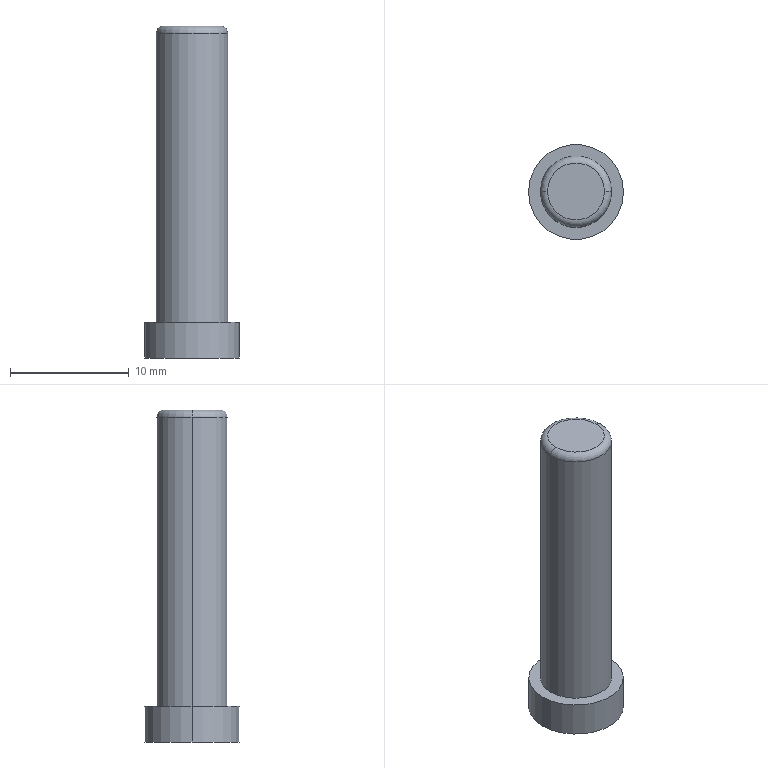Part | SolidWorks | features BaseBody 1 | 1 solid | 9 faces | box 8 x 8 x 28 mm | volume 856.499 mm3 | cylinder 4 | plane 3 | torus 2 | commonest cylinder face diameters 6.001 x2 8 x2
STEP:
#1=CARTESIAN_POINT('',(-82.,-25.,-3.829));
#2=VERTEX_POINT('',#1);
#3=CARTESIAN_POINT('',(-90.,-25.,-3.829));
#4=VERTEX_POINT('',#3);
#5=CARTESIAN_POINT('',(-86.,-25.,-3.829));
#6=DIRECTION('',(0.,0.,-1.));
#7=DIRECTION('',(1.,0.,0.));
#8=AXIS2_PLACEMENT_3D('',#5,#6,#7);
#9=CIRCLE('',#8,4.);
#10=EDGE_CURVE('',#2,#4,#9,.T.);
#11=ORIENTED_EDGE('',*,*,#10,.T.);
#12=CARTESIAN_POINT('',(-90.,-25.,-6.829));
#13=VERTEX_POINT('',#12);
#14=CARTESIAN_POINT('',(-90.,-25.,-3.829));
#15=DIRECTION('',(0.,0.,-1.));
#16=VECTOR('',#15,1000.);
#17=LINE('',#14,#16);
#18=EDGE_CURVE('',#4,#13,#17,.T.);
#19=ORIENTED_EDGE('',*,*,#18,.T.);
#20=CARTESIAN_POINT('',(-82.,-25.,-6.829));
#21=VERTEX_POINT('',#20);
#22=CARTESIAN_POINT('',(-86.,-25.,-6.829));
#23=DIRECTION('',(0.,0.,1.));
#24=DIRECTION('',(1.,0.,0.));
#25=AXIS2_PLACEMENT_3D('',#22,#23,#24);
#26=CIRCLE('',#25,4.);
#27=EDGE_CURVE('',#13,#21,#26,.T.);
#28=ORIENTED_EDGE('',*,*,#27,.T.);
#29=CARTESIAN_POINT('',(-82.,-25.,-3.829));
#30=DIRECTION('',(0.,0.,-1.));
#31=VECTOR('',#30,1000.);
#32=LINE('',#29,#31);
#33=EDGE_CURVE('',#2,#21,#32,.T.);
#34=ORIENTED_EDGE('',*,*,#33,.F.);
#35=EDGE_LOOP('',(#11,#19,#28,#34));
#36=FACE_OUTER_BOUND('',#35,.T.);
#37=CARTESIAN_POINT('',(-86.,-25.,-3.829));
#38=DIRECTION('',(0.,0.,-1.));
#39=DIRECTION('',(1.,0.,0.));
#40=AXIS2_PLACEMENT_3D('',#37,#38,#39);
#41=CYLINDRICAL_SURFACE('',#40,4.);
#42=ADVANCED_FACE('',(#36),#41,.T.);
#43=CARTESIAN_POINT('',(-89.001,-25.,20.571));
#44=VERTEX_POINT('',#43);
#45=CARTESIAN_POINT('',(-82.999,-25.,20.571));
#46=VERTEX_POINT('',#45);
#47=CARTESIAN_POINT('',(-86.,-25.,20.571));
#48=DIRECTION('',(0.,0.,-1.));
#49=DIRECTION('',(1.,0.,0.));
#50=AXIS2_PLACEMENT_3D('',#47,#48,#49);
#51=CIRCLE('',#50,3.001);
#52=EDGE_CURVE('',#44,#46,#51,.T.);
#53=ORIENTED_EDGE('',*,*,#52,.F.);
#54=CARTESIAN_POINT('',(-88.4,-25.,21.171));
#55=VERTEX_POINT('',#54);
#56=CARTESIAN_POINT('',(-88.4,-25.,20.571));
#57=DIRECTION('',(0.,1.,0.));
#58=DIRECTION('',(-1.,0.,0.));
#59=AXIS2_PLACEMENT_3D('',#56,#57,#58);
#60=CIRCLE('',#59,0.6001);
#61=EDGE_CURVE('',#44,#55,#60,.T.);
#62=ORIENTED_EDGE('',*,*,#61,.T.);
#63=CARTESIAN_POINT('',(-83.6,-25.,21.171));
#64=VERTEX_POINT('',#63);
#65=CARTESIAN_POINT('',(-86.,-25.,21.171));
#66=DIRECTION('',(0.,0.,1.));
#67=DIRECTION('',(1.,0.,0.));
#68=AXIS2_PLACEMENT_3D('',#65,#66,#67);
#69=CIRCLE('',#68,2.4);
#70=EDGE_CURVE('',#64,#55,#69,.T.);
#71=ORIENTED_EDGE('',*,*,#70,.F.);
#72=CARTESIAN_POINT('',(-83.6,-25.,20.571));
#73=DIRECTION('',(0.,-1.,0.));
#74=DIRECTION('',(0.,0.,-1.));
#75=AXIS2_PLACEMENT_3D('',#72,#73,#74);
#76=CIRCLE('',#75,0.6001);
#77=EDGE_CURVE('',#46,#64,#76,.T.);
#78=ORIENTED_EDGE('',*,*,#77,.F.);
#79=EDGE_LOOP('',(#53,#62,#71,#78));
#80=FACE_OUTER_BOUND('',#79,.T.);
#81=CARTESIAN_POINT('',(-86.,-25.,20.571));
#82=DIRECTION('',(0.,0.,1.));
#83=DIRECTION('',(1.,0.,0.));
#84=AXIS2_PLACEMENT_3D('',#81,#82,#83);
#85=TOROIDAL_SURFACE('',#84,2.4,0.6001);
#86=ADVANCED_FACE('',(#80),#85,.T.);
#87=CARTESIAN_POINT('',(-86.,-25.,20.571));
#88=DIRECTION('',(0.,0.,-1.));
#89=DIRECTION('',(1.,0.,0.));
#90=AXIS2_PLACEMENT_3D('',#87,#88,#89);
#91=CIRCLE('',#90,3.001);
#92=EDGE_CURVE('',#46,#44,#91,.T.);
#93=ORIENTED_EDGE('',*,*,#92,.T.);
#94=CARTESIAN_POINT('',(-89.001,-25.,-3.829));
#95=VERTEX_POINT('',#94);
#96=CARTESIAN_POINT('',(-89.001,-25.,21.171));
#97=DIRECTION('',(0.,0.,-1.));
#98=VECTOR('',#97,1000.);
#99=LINE('',#96,#98);
#100=EDGE_CURVE('',#44,#95,#99,.T.);
#101=ORIENTED_EDGE('',*,*,#100,.T.);
#102=CARTESIAN_POINT('',(-82.999,-25.,-3.829));
#103=VERTEX_POINT('',#102);
#104=CARTESIAN_POINT('',(-86.,-25.,-3.829));
#105=DIRECTION('',(0.,0.,1.));
#106=DIRECTION('',(1.,0.,0.));
#107=AXIS2_PLACEMENT_3D('',#104,#105,#106);
#108=CIRCLE('',#107,3.001);
#109=EDGE_CURVE('',#95,#103,#108,.T.);
#110=ORIENTED_EDGE('',*,*,#109,.T.);
#111=CARTESIAN_POINT('',(-82.999,-25.,21.171));
#112=DIRECTION('',(0.,0.,-1.));
#113=VECTOR('',#112,1000.);
#114=LINE('',#111,#113);
#115=EDGE_CURVE('',#46,#103,#114,.T.);
#116=ORIENTED_EDGE('',*,*,#115,.F.);
#117=EDGE_LOOP('',(#93,#101,#110,#116));
#118=FACE_OUTER_BOUND('',#117,.T.);
#119=CARTESIAN_POINT('',(-86.,-25.,21.171));
#120=DIRECTION('',(0.,0.,-1.));
#121=DIRECTION('',(1.,0.,0.));
#122=AXIS2_PLACEMENT_3D('',#119,#120,#121);
#123=CYLINDRICAL_SURFACE('',#122,3.001);
#124=ADVANCED_FACE('',(#118),#123,.T.);
#125=ORIENTED_EDGE('',*,*,#70,.T.);
#126=CARTESIAN_POINT('',(-86.,-25.,21.171));
#127=DIRECTION('',(0.,0.,1.));
#128=DIRECTION('',(1.,0.,0.));
#129=AXIS2_PLACEMENT_3D('',#126,#127,#128);
#130=CIRCLE('',#129,2.4);
#131=EDGE_CURVE('',#55,#64,#130,.T.);
#132=ORIENTED_EDGE('',*,*,#131,.T.);
#133=EDGE_LOOP('',(#125,#132));
#134=FACE_OUTER_BOUND('',#133,.T.);
#135=CARTESIAN_POINT('',(-86.,-25.,21.171));
#136=DIRECTION('',(0.,0.,1.));
#137=DIRECTION('',(1.,0.,0.));
#138=AXIS2_PLACEMENT_3D('',#135,#136,#137);
#139=PLANE('',#138);
#140=ADVANCED_FACE('',(#134),#139,.T.);
#141=ORIENTED_EDGE('',*,*,#100,.F.);
#142=ORIENTED_EDGE('',*,*,#52,.T.);
#143=ORIENTED_EDGE('',*,*,#115,.T.);
#144=CARTESIAN_POINT('',(-86.,-25.,-3.829));
#145=DIRECTION('',(0.,0.,1.));
#146=DIRECTION('',(1.,0.,0.));
#147=AXIS2_PLACEMENT_3D('',#144,#145,#146);
#148=CIRCLE('',#147,3.001);
#149=EDGE_CURVE('',#103,#95,#148,.T.);
#150=ORIENTED_EDGE('',*,*,#149,.T.);
#151=EDGE_LOOP('',(#141,#142,#143,#150));
#152=FACE_OUTER_BOUND('',#151,.T.);
#153=CARTESIAN_POINT('',(-86.,-25.,21.171));
#154=DIRECTION('',(0.,0.,-1.));
#155=DIRECTION('',(1.,0.,0.));
#156=AXIS2_PLACEMENT_3D('',#153,#154,#155);
#157=CYLINDRICAL_SURFACE('',#156,3.001);
#158=ADVANCED_FACE('',(#152),#157,.T.);
#159=ORIENTED_EDGE('',*,*,#61,.F.);
#160=ORIENTED_EDGE('',*,*,#92,.F.);
#161=ORIENTED_EDGE('',*,*,#77,.T.);
#162=ORIENTED_EDGE('',*,*,#131,.F.);
#163=EDGE_LOOP('',(#159,#160,#161,#162));
#164=FACE_OUTER_BOUND('',#163,.T.);
#165=CARTESIAN_POINT('',(-86.,-25.,20.571));
#166=DIRECTION('',(0.,0.,1.));
#167=DIRECTION('',(1.,0.,0.));
#168=AXIS2_PLACEMENT_3D('',#165,#166,#167);
#169=TOROIDAL_SURFACE('',#168,2.4,0.6001);
#170=ADVANCED_FACE('',(#164),#169,.T.);
#171=CARTESIAN_POINT('',(-86.,-25.,-6.829));
#172=DIRECTION('',(0.,0.,1.));
#173=DIRECTION('',(1.,0.,0.));
#174=AXIS2_PLACEMENT_3D('',#171,#172,#173);
#175=CIRCLE('',#174,4.);
#176=EDGE_CURVE('',#21,#13,#175,.T.);
#177=ORIENTED_EDGE('',*,*,#176,.F.);
#178=ORIENTED_EDGE('',*,*,#27,.F.);
#179=EDGE_LOOP('',(#177,#178));
#180=FACE_OUTER_BOUND('',#179,.T.);
#181=CARTESIAN_POINT('',(-86.,-25.,-6.829));
#182=DIRECTION('',(0.,0.,-1.));
#183=DIRECTION('',(-1.,0.,0.));
#184=AXIS2_PLACEMENT_3D('',#181,#182,#183);
#185=PLANE('',#184);
#186=ADVANCED_FACE('',(#180),#185,.T.);
#187=ORIENTED_EDGE('',*,*,#149,.F.);
#188=ORIENTED_EDGE('',*,*,#109,.F.);
#189=EDGE_LOOP('',(#187,#188));
#190=FACE_BOUND('',#189,.T.);
#191=ORIENTED_EDGE('',*,*,#10,.F.);
#192=CARTESIAN_POINT('',(-86.,-25.,-3.829));
#193=DIRECTION('',(0.,0.,-1.));
#194=DIRECTION('',(1.,0.,0.));
#195=AXIS2_PLACEMENT_3D('',#192,#193,#194);
#196=CIRCLE('',#195,4.);
#197=EDGE_CURVE('',#4,#2,#196,.T.);
#198=ORIENTED_EDGE('',*,*,#197,.F.);
#199=EDGE_LOOP('',(#191,#198));
#200=FACE_OUTER_BOUND('',#199,.T.);
#201=CARTESIAN_POINT('',(-86.,-25.,-3.829));
#202=DIRECTION('',(0.,0.,1.));
#203=DIRECTION('',(1.,0.,0.));
#204=AXIS2_PLACEMENT_3D('',#201,#202,#203);
#205=PLANE('',#204);
#206=ADVANCED_FACE('',(#190,#200),#205,.T.);
#207=ORIENTED_EDGE('',*,*,#18,.F.);
#208=ORIENTED_EDGE('',*,*,#197,.T.);
#209=ORIENTED_EDGE('',*,*,#33,.T.);
#210=ORIENTED_EDGE('',*,*,#176,.T.);
#211=EDGE_LOOP('',(#207,#208,#209,#210));
#212=FACE_OUTER_BOUND('',#211,.T.);
#213=CARTESIAN_POINT('',(-86.,-25.,-3.829));
#214=DIRECTION('',(0.,0.,-1.));
#215=DIRECTION('',(1.,0.,0.));
#216=AXIS2_PLACEMENT_3D('',#213,#214,#215);
#217=CYLINDRICAL_SURFACE('',#216,4.);
#218=ADVANCED_FACE('',(#212),#217,.T.);
#219=CLOSED_SHELL('',(#42,#86,#124,#140,#158,#170,#186,#206,#218));
#220=MANIFOLD_SOLID_BREP('',#219);
#221=CARTESIAN_POINT('',(0.,0.,0.));
#222=DIRECTION('',(0.,0.,1.));
#223=DIRECTION('',(1.,0.,0.));
#224=AXIS2_PLACEMENT_3D('',#221,#222,#223);
#225=(LENGTH_UNIT()NAMED_UNIT(*)SI_UNIT(.MILLI.,.METRE.));
#226=UNCERTAINTY_MEASURE_WITH_UNIT(LENGTH_MEASURE(0.00001),#225,'','');
#227=(NAMED_UNIT(*)PLANE_ANGLE_UNIT()SI_UNIT($,.RADIAN.));
#228=(NAMED_UNIT(*)SI_UNIT($,.STERADIAN.)SOLID_ANGLE_UNIT());
#229=(GEOMETRIC_REPRESENTATION_CONTEXT(3)GLOBAL_UNCERTAINTY_ASSIGNED_CONTEXT((#226))GLOBAL_UNIT_ASSIGNED_CONTEXT((#225,#227,#228))REPRESENTATION_CONTEXT('',''));
#230=ADVANCED_BREP_SHAPE_REPRESENTATION('',(#220,#224),#229);